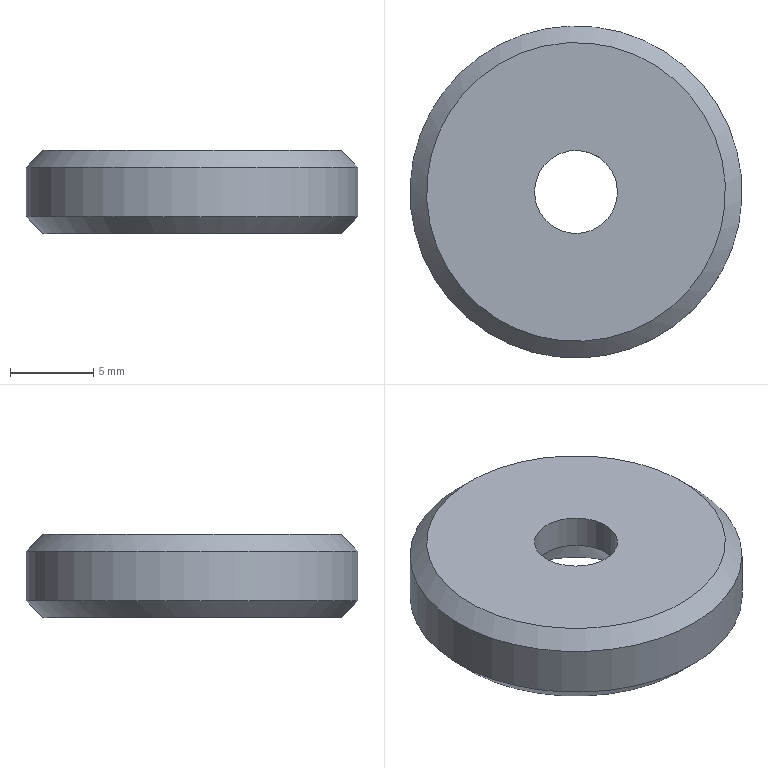Part | STEP file | stop_rings_id14_x_t | 1 solid | 7 faces | box 20 x 20 x 5 mm | volume 1313 mm3 | cone 3 | cylinder 2 | plane 2 | commonest cylinder face diameters 5 x1 20 x1
STEP:
#1=CARTESIAN_POINT('',(128.387,250.425,-369.5));
#2=VERTEX_POINT('',#1);
#3=CARTESIAN_POINT('',(123.,242.,-369.5));
#4=DIRECTION('',(0.,0.,1.));
#5=DIRECTION('',(0.5387,0.8425,0.));
#6=AXIS2_PLACEMENT_3D('',#3,#4,#5);
#7=CIRCLE('',#6,10.);
#8=EDGE_CURVE('',#2,#2,#7,.T.);
#9=ORIENTED_EDGE('',*,*,#8,.T.);
#10=EDGE_LOOP('',(#9));
#11=FACE_BOUND('',#10,.T.);
#12=CARTESIAN_POINT('',(128.387,250.425,-366.5));
#13=VERTEX_POINT('',#12);
#14=CARTESIAN_POINT('',(123.,242.,-366.5));
#15=DIRECTION('',(0.,0.,-1.));
#16=DIRECTION('',(0.5387,0.8425,0.));
#17=AXIS2_PLACEMENT_3D('',#14,#15,#16);
#18=CIRCLE('',#17,10.);
#19=EDGE_CURVE('',#13,#13,#18,.T.);
#20=ORIENTED_EDGE('',*,*,#19,.T.);
#21=EDGE_LOOP('',(#20));
#22=FACE_BOUND('',#21,.T.);
#23=CARTESIAN_POINT('',(123.,242.,-370.5));
#24=DIRECTION('',(0.,0.,1.));
#25=DIRECTION('',(-0.5387,-0.8425,0.));
#26=AXIS2_PLACEMENT_3D('',#23,#24,#25);
#27=CYLINDRICAL_SURFACE('',#26,10.);
#28=ADVANCED_FACE('',(#11,#22),#27,.T.);
#29=CARTESIAN_POINT('',(127.848,249.583,-370.5));
#30=VERTEX_POINT('',#29);
#31=CARTESIAN_POINT('',(123.,242.,-370.5));
#32=DIRECTION('',(0.,0.,-1.));
#33=DIRECTION('',(0.5387,0.8425,0.));
#34=AXIS2_PLACEMENT_3D('',#31,#32,#33);
#35=CIRCLE('',#34,9.);
#36=EDGE_CURVE('',#30,#30,#35,.T.);
#37=ORIENTED_EDGE('',*,*,#36,.T.);
#38=EDGE_LOOP('',(#37));
#39=FACE_BOUND('',#38,.T.);
#40=CARTESIAN_POINT('',(125.963,246.634,-370.5));
#41=VERTEX_POINT('',#40);
#42=CARTESIAN_POINT('',(123.,242.,-370.5));
#43=DIRECTION('',(0.,0.,-1.));
#44=DIRECTION('',(0.5387,0.8425,0.));
#45=AXIS2_PLACEMENT_3D('',#42,#43,#44);
#46=CIRCLE('',#45,5.5);
#47=EDGE_CURVE('',#41,#41,#46,.T.);
#48=ORIENTED_EDGE('',*,*,#47,.F.);
#49=EDGE_LOOP('',(#48));
#50=FACE_BOUND('',#49,.T.);
#51=CARTESIAN_POINT('',(123.,242.,-370.5));
#52=DIRECTION('',(0.,0.,-1.));
#53=DIRECTION('',(0.5387,0.8425,0.));
#54=AXIS2_PLACEMENT_3D('',#51,#52,#53);
#55=PLANE('',#54);
#56=ADVANCED_FACE('',(#39,#50),#55,.T.);
#57=CARTESIAN_POINT('',(127.848,249.583,-365.5));
#58=VERTEX_POINT('',#57);
#59=CARTESIAN_POINT('',(123.,242.,-365.5));
#60=DIRECTION('',(0.,0.,1.));
#61=DIRECTION('',(0.5387,0.8425,0.));
#62=AXIS2_PLACEMENT_3D('',#59,#60,#61);
#63=CIRCLE('',#62,9.);
#64=EDGE_CURVE('',#58,#58,#63,.T.);
#65=ORIENTED_EDGE('',*,*,#64,.T.);
#66=EDGE_LOOP('',(#65));
#67=FACE_BOUND('',#66,.T.);
#68=CARTESIAN_POINT('',(124.347,244.106,-365.5));
#69=VERTEX_POINT('',#68);
#70=CARTESIAN_POINT('',(123.,242.,-365.5));
#71=DIRECTION('',(0.,0.,-1.));
#72=DIRECTION('',(0.5387,0.8425,0.));
#73=AXIS2_PLACEMENT_3D('',#70,#71,#72);
#74=CIRCLE('',#73,2.5);
#75=EDGE_CURVE('',#69,#69,#74,.T.);
#76=ORIENTED_EDGE('',*,*,#75,.T.);
#77=EDGE_LOOP('',(#76));
#78=FACE_BOUND('',#77,.T.);
#79=CARTESIAN_POINT('',(123.,242.,-365.5));
#80=DIRECTION('',(0.,0.,-1.));
#81=DIRECTION('',(0.5387,0.8425,0.));
#82=AXIS2_PLACEMENT_3D('',#79,#80,#81);
#83=PLANE('',#82);
#84=ADVANCED_FACE('',(#67,#78),#83,.F.);
#85=CARTESIAN_POINT('',(124.347,244.106,-367.5));
#86=VERTEX_POINT('',#85);
#87=CARTESIAN_POINT('',(123.,242.,-367.5));
#88=DIRECTION('',(0.,0.,-1.));
#89=DIRECTION('',(0.5387,0.8425,0.));
#90=AXIS2_PLACEMENT_3D('',#87,#88,#89);
#91=CIRCLE('',#90,2.5);
#92=EDGE_CURVE('',#86,#86,#91,.T.);
#93=ORIENTED_EDGE('',*,*,#92,.F.);
#94=EDGE_LOOP('',(#93));
#95=FACE_BOUND('',#94,.T.);
#96=ORIENTED_EDGE('',*,*,#47,.T.);
#97=EDGE_LOOP('',(#96));
#98=FACE_BOUND('',#97,.T.);
#99=CARTESIAN_POINT('',(123.,242.,-370.5));
#100=DIRECTION('',(0.,0.,-1.));
#101=DIRECTION('',(0.5387,0.8425,0.));
#102=AXIS2_PLACEMENT_3D('',#99,#100,#101);
#103=CONICAL_SURFACE('',#102,5.5,45.);
#104=ADVANCED_FACE('',(#95,#98),#103,.F.);
#105=ORIENTED_EDGE('',*,*,#75,.F.);
#106=EDGE_LOOP('',(#105));
#107=FACE_BOUND('',#106,.T.);
#108=ORIENTED_EDGE('',*,*,#92,.T.);
#109=EDGE_LOOP('',(#108));
#110=FACE_BOUND('',#109,.T.);
#111=CARTESIAN_POINT('',(123.,242.,-375.095));
#112=DIRECTION('',(0.,0.,-1.));
#113=DIRECTION('',(0.5387,0.8425,0.));
#114=AXIS2_PLACEMENT_3D('',#111,#112,#113);
#115=CYLINDRICAL_SURFACE('',#114,2.5);
#116=ADVANCED_FACE('',(#107,#110),#115,.F.);
#117=ORIENTED_EDGE('',*,*,#8,.F.);
#118=EDGE_LOOP('',(#117));
#119=FACE_BOUND('',#118,.T.);
#120=ORIENTED_EDGE('',*,*,#36,.F.);
#121=EDGE_LOOP('',(#120));
#122=FACE_BOUND('',#121,.T.);
#123=CARTESIAN_POINT('',(123.,242.,-370.5));
#124=DIRECTION('',(0.,0.,1.));
#125=DIRECTION('',(-0.5387,-0.8425,0.));
#126=AXIS2_PLACEMENT_3D('',#123,#124,#125);
#127=CONICAL_SURFACE('',#126,9.,45.);
#128=ADVANCED_FACE('',(#119,#122),#127,.T.);
#129=ORIENTED_EDGE('',*,*,#64,.F.);
#130=EDGE_LOOP('',(#129));
#131=FACE_BOUND('',#130,.T.);
#132=ORIENTED_EDGE('',*,*,#19,.F.);
#133=EDGE_LOOP('',(#132));
#134=FACE_BOUND('',#133,.T.);
#135=CARTESIAN_POINT('',(123.,242.,-366.5));
#136=DIRECTION('',(0.,0.,-1.));
#137=DIRECTION('',(0.5387,0.8425,0.));
#138=AXIS2_PLACEMENT_3D('',#135,#136,#137);
#139=CONICAL_SURFACE('',#138,10.,45.);
#140=ADVANCED_FACE('',(#131,#134),#139,.T.);
#141=CLOSED_SHELL('',(#28,#56,#84,#104,#116,#128,#140));
#142=MANIFOLD_SOLID_BREP('',#141);
#143=(LENGTH_UNIT()NAMED_UNIT(*)SI_UNIT(.MILLI.,.METRE.));
#144=UNCERTAINTY_MEASURE_WITH_UNIT(LENGTH_MEASURE(0.00002),#143,'','');
#145=(NAMED_UNIT(*)PLANE_ANGLE_UNIT()SI_UNIT($,.RADIAN.));
#146=PLANE_ANGLE_MEASURE_WITH_UNIT(PLANE_ANGLE_MEASURE(0.01745),#145);
#147=DIMENSIONAL_EXPONENTS(0.,0.,0.,0.,0.,0.,0.);
#148=(CONVERSION_BASED_UNIT('DEGREE',#146)NAMED_UNIT(#147)PLANE_ANGLE_UNIT());
#149=(NAMED_UNIT(*)SI_UNIT($,.STERADIAN.)SOLID_ANGLE_UNIT());
#150=(GEOMETRIC_REPRESENTATION_CONTEXT(3)GLOBAL_UNCERTAINTY_ASSIGNED_CONTEXT((#144))GLOBAL_UNIT_ASSIGNED_CONTEXT((#143,#148,#149))REPRESENTATION_CONTEXT('',''));
#151=ADVANCED_BREP_SHAPE_REPRESENTATION('',(#142),#150);